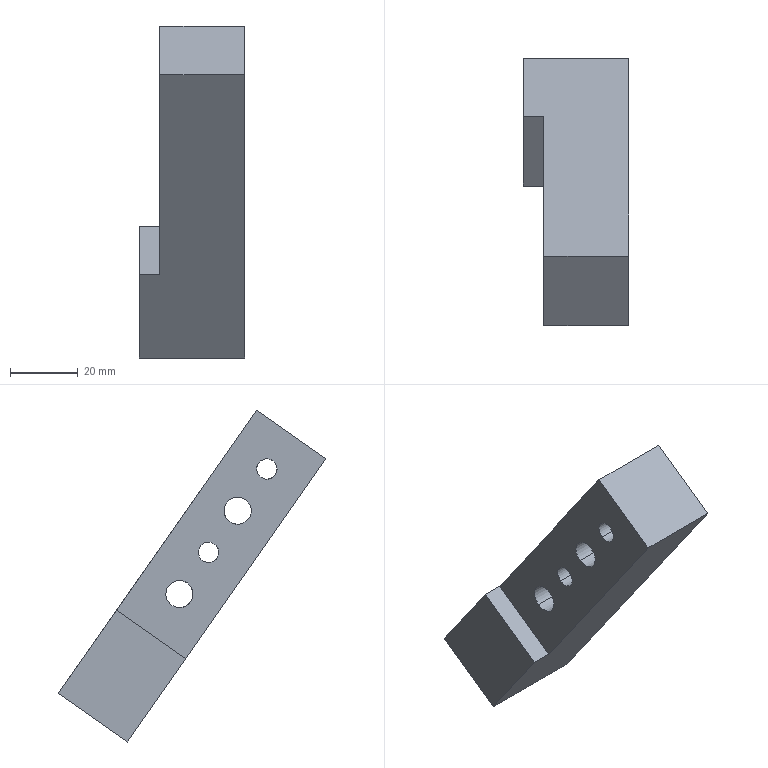Part | STEP file | Positioning_id1782_x_t | 1 solid | 16 faces | box 30.998 x 78.984 x 97.893 mm | volume 64322 mm3 | plane 8 | cylinder 8 | commonest cylinder face diameters 6 x4 8 x4